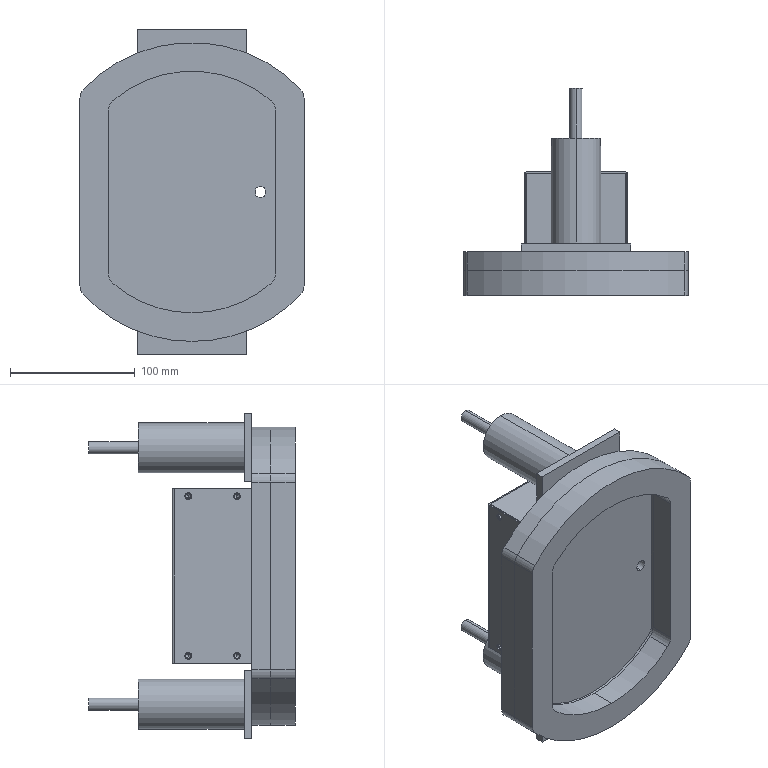Part | SolidWorks | features InContextFeatHolder 4 | 12 solids | 453 faces | box 180 x 166 x 261 mm | volume 1533619 mm3 | cylinder 253 | plane 110 | cone 90 | commonest cylinder face diameters 4.2 x60 5.5 x48 10 x20 1.6 x16 3.4 x16 20 x16